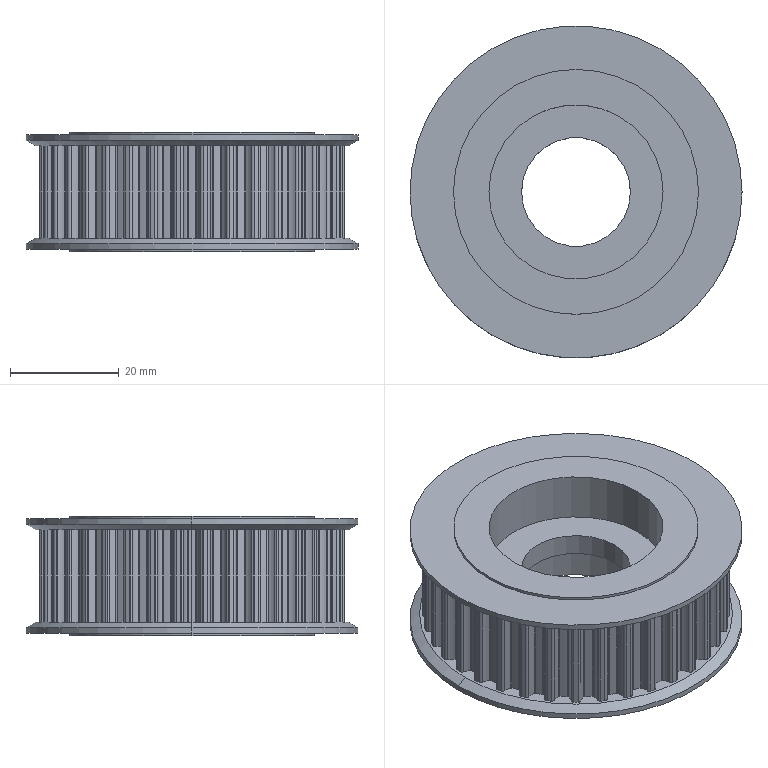Part | STEP file | Y-EAB01-S5M150-36-A-H-d28 tube-turning tensioning pulley SGN-2-18 | 1 solid | 347 faces | box 61 x 61 x 22 mm | volume 36726 mm3 | cylinder 335 | plane 8 | cone 4 | commonest cylinder face diameters 1 x88 0.5 x82 6.55 x78 52.8 x37 56.34 x36 32 x4